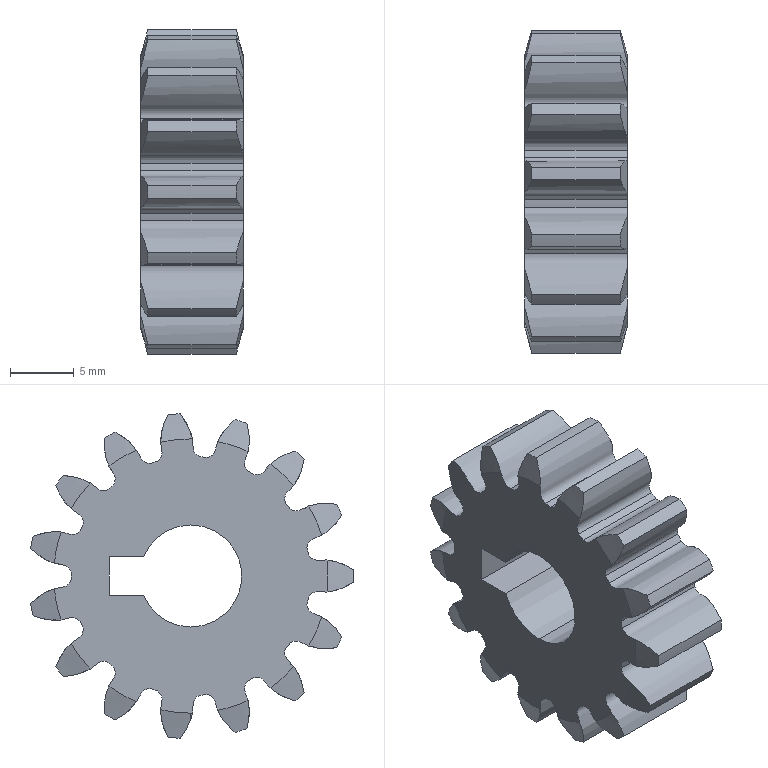Part | SolidWorks | features Chamfer 2, ICE 2, CirPattern 1, Extrusion 1, RefAxis 1 | 1 solid | 100 faces | box 8 x 25.314 x 25.444 mm | volume 2620 mm3 | cylinder 33 | cone 32 | spline 30 | plane 5 | commonest cylinder face diameters 18.75 x15 25.5 x15 8 x3